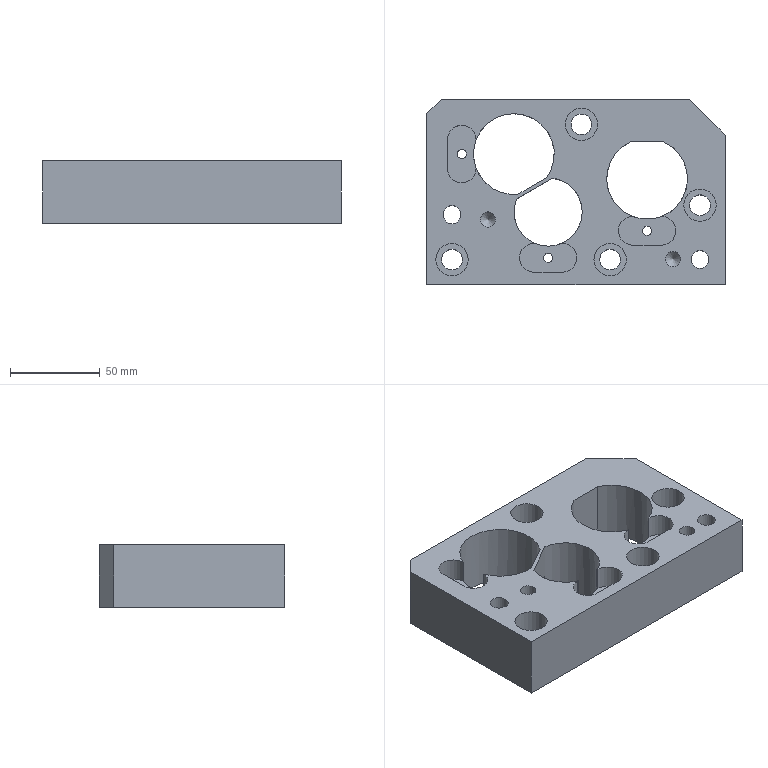Part | STEP file | lll_id4570_x_t | 1 solid | 49 faces | box 166 x 103.25 x 35 mm | volume 394773 mm3 | cylinder 24 | plane 23 | cone 2 | commonest cylinder face diameters 16 x6 11.509 x4 18.008 x4 5.206 x3 8.506 x2 10 x2
STEP:
#1=CARTESIAN_POINT('',(3308.367,-51.288,0.));
#2=VERTEX_POINT('',#1);
#3=CARTESIAN_POINT('',(3324.366,-51.364,0.));
#4=VERTEX_POINT('',#3);
#5=CARTESIAN_POINT('',(3316.367,-51.288,0.));
#6=DIRECTION('',(0.,0.,1.));
#7=DIRECTION('',(1.,0.,0.));
#8=AXIS2_PLACEMENT_3D('',#5,#6,#7);
#9=CIRCLE('',#8,8.);
#10=EDGE_CURVE('',#2,#4,#9,.T.);
#11=ORIENTED_EDGE('',*,*,#10,.F.);
#12=CARTESIAN_POINT('',(3308.367,-35.288,0.));
#13=VERTEX_POINT('',#12);
#14=CARTESIAN_POINT('',(3308.367,-54.25,0.));
#15=DIRECTION('',(0.,1.,0.));
#16=VECTOR('',#15,1.);
#17=LINE('',#14,#16);
#18=EDGE_CURVE('',#2,#13,#17,.T.);
#19=ORIENTED_EDGE('',*,*,#18,.T.);
#20=CARTESIAN_POINT('',(3324.366,-35.211,0.));
#21=VERTEX_POINT('',#20);
#22=CARTESIAN_POINT('',(3316.367,-35.288,0.));
#23=DIRECTION('',(0.,0.,1.));
#24=DIRECTION('',(1.,0.,0.));
#25=AXIS2_PLACEMENT_3D('',#22,#23,#24);
#26=CIRCLE('',#25,8.);
#27=EDGE_CURVE('',#21,#13,#26,.T.);
#28=ORIENTED_EDGE('',*,*,#27,.F.);
#29=CARTESIAN_POINT('',(3363.648,-56.404,0.));
#30=VERTEX_POINT('',#29);
#31=CARTESIAN_POINT('',(3345.367,-43.288,0.));
#32=DIRECTION('',(0.,0.,1.));
#33=DIRECTION('',(1.,0.,0.));
#34=AXIS2_PLACEMENT_3D('',#31,#32,#33);
#35=CIRCLE('',#34,22.5);
#36=EDGE_CURVE('',#30,#21,#35,.T.);
#37=ORIENTED_EDGE('',*,*,#36,.F.);
#38=CARTESIAN_POINT('',(3347.585,-65.678,0.));
#39=VERTEX_POINT('',#38);
#40=CARTESIAN_POINT('',(3355.617,-61.041,0.));
#41=DIRECTION('',(-0.866,-0.5,0.));
#42=VECTOR('',#41,1.);
#43=LINE('',#40,#42);
#44=EDGE_CURVE('',#30,#39,#43,.T.);
#45=ORIENTED_EDGE('',*,*,#44,.T.);
#46=CARTESIAN_POINT('',(3345.367,-43.288,0.));
#47=DIRECTION('',(0.,0.,1.));
#48=DIRECTION('',(1.,0.,0.));
#49=AXIS2_PLACEMENT_3D('',#46,#47,#48);
#50=CIRCLE('',#49,22.5);
#51=EDGE_CURVE('',#4,#39,#50,.T.);
#52=ORIENTED_EDGE('',*,*,#51,.F.);
#53=EDGE_LOOP('',(#11,#19,#28,#37,#45,#52));
#54=FACE_BOUND('',#53,.T.);
#55=CARTESIAN_POINT('',(3442.935,-12.75,0.));
#56=VERTEX_POINT('',#55);
#57=CARTESIAN_POINT('',(3304.935,-12.75,0.));
#58=VERTEX_POINT('',#57);
#59=CARTESIAN_POINT('',(3266.435,-12.75,0.));
#60=DIRECTION('',(-1.,0.,0.));
#61=VECTOR('',#60,1.);
#62=LINE('',#59,#61);
#63=EDGE_CURVE('',#56,#58,#62,.T.);
#64=ORIENTED_EDGE('',*,*,#63,.T.);
#65=CARTESIAN_POINT('',(3296.935,-20.75,0.));
#66=VERTEX_POINT('',#65);
#67=CARTESIAN_POINT('',(3179.435,-138.25,0.));
#68=DIRECTION('',(0.7071,0.7071,0.));
#69=VECTOR('',#68,1.);
#70=LINE('',#67,#69);
#71=EDGE_CURVE('',#66,#58,#70,.T.);
#72=ORIENTED_EDGE('',*,*,#71,.F.);
#73=CARTESIAN_POINT('',(3296.935,-116.,0.));
#74=VERTEX_POINT('',#73);
#75=CARTESIAN_POINT('',(3296.935,-215.25,0.));
#76=DIRECTION('',(0.,1.,0.));
#77=VECTOR('',#76,1.);
#78=LINE('',#75,#77);
#79=EDGE_CURVE('',#74,#66,#78,.T.);
#80=ORIENTED_EDGE('',*,*,#79,.F.);
#81=CARTESIAN_POINT('',(3462.935,-116.,0.));
#82=VERTEX_POINT('',#81);
#83=CARTESIAN_POINT('',(3266.435,-116.,0.));
#84=DIRECTION('',(-1.,0.,0.));
#85=VECTOR('',#84,1.);
#86=LINE('',#83,#85);
#87=EDGE_CURVE('',#82,#74,#86,.T.);
#88=ORIENTED_EDGE('',*,*,#87,.F.);
#89=CARTESIAN_POINT('',(3462.935,-32.75,0.));
#90=VERTEX_POINT('',#89);
#91=CARTESIAN_POINT('',(3462.935,-215.25,0.));
#92=DIRECTION('',(0.,1.,0.));
#93=VECTOR('',#92,1.);
#94=LINE('',#91,#93);
#95=EDGE_CURVE('',#82,#90,#94,.T.);
#96=ORIENTED_EDGE('',*,*,#95,.T.);
#97=CARTESIAN_POINT('',(3455.935,-25.75,0.));
#98=DIRECTION('',(0.7071,-0.7071,0.));
#99=VECTOR('',#98,1.);
#100=LINE('',#97,#99);
#101=EDGE_CURVE('',#56,#90,#100,.T.);
#102=ORIENTED_EDGE('',*,*,#101,.F.);
#103=EDGE_LOOP('',(#64,#72,#80,#88,#96,#102));
#104=FACE_BOUND('',#103,.T.);
#105=CARTESIAN_POINT('',(3319.939,-102.,0.));
#106=VERTEX_POINT('',#105);
#107=CARTESIAN_POINT('',(3310.935,-102.,0.));
#108=DIRECTION('',(0.,0.,-1.));
#109=DIRECTION('',(1.,0.,0.));
#110=AXIS2_PLACEMENT_3D('',#107,#108,#109);
#111=CIRCLE('',#110,9.004);
#112=EDGE_CURVE('',#106,#106,#111,.T.);
#113=ORIENTED_EDGE('',*,*,#112,.T.);
#114=EDGE_LOOP('',(#113));
#115=FACE_BOUND('',#114,.T.);
#116=CARTESIAN_POINT('',(3315.935,-77.,0.));
#117=VERTEX_POINT('',#116);
#118=CARTESIAN_POINT('',(3310.935,-77.,0.));
#119=DIRECTION('',(0.,0.,-1.));
#120=DIRECTION('',(1.,0.,0.));
#121=AXIS2_PLACEMENT_3D('',#118,#119,#120);
#122=CIRCLE('',#121,5.);
#123=EDGE_CURVE('',#117,#117,#122,.T.);
#124=ORIENTED_EDGE('',*,*,#123,.T.);
#125=EDGE_LOOP('',(#124));
#126=FACE_BOUND('',#125,.T.);
#127=CARTESIAN_POINT('',(3335.188,-79.75,0.));
#128=VERTEX_POINT('',#127);
#129=CARTESIAN_POINT('',(3330.935,-79.75,0.));
#130=DIRECTION('',(0.,0.,-1.));
#131=DIRECTION('',(1.,0.,0.));
#132=AXIS2_PLACEMENT_3D('',#129,#130,#131);
#133=CIRCLE('',#132,4.253);
#134=EDGE_CURVE('',#128,#128,#133,.T.);
#135=ORIENTED_EDGE('',*,*,#134,.T.);
#136=EDGE_LOOP('',(#135));
#137=FACE_BOUND('',#136,.T.);
#138=CARTESIAN_POINT('',(3391.939,-26.75,0.));
#139=VERTEX_POINT('',#138);
#140=CARTESIAN_POINT('',(3382.935,-26.75,0.));
#141=DIRECTION('',(0.,0.,-1.));
#142=DIRECTION('',(1.,0.,0.));
#143=AXIS2_PLACEMENT_3D('',#140,#141,#142);
#144=CIRCLE('',#143,9.004);
#145=EDGE_CURVE('',#139,#139,#144,.T.);
#146=ORIENTED_EDGE('',*,*,#145,.T.);
#147=EDGE_LOOP('',(#146));
#148=FACE_BOUND('',#147,.T.);
#149=CARTESIAN_POINT('',(3457.939,-71.75,0.));
#150=VERTEX_POINT('',#149);
#151=CARTESIAN_POINT('',(3448.935,-71.75,0.));
#152=DIRECTION('',(0.,0.,-1.));
#153=DIRECTION('',(1.,0.,0.));
#154=AXIS2_PLACEMENT_3D('',#151,#152,#153);
#155=CIRCLE('',#154,9.004);
#156=EDGE_CURVE('',#150,#150,#155,.T.);
#157=ORIENTED_EDGE('',*,*,#156,.T.);
#158=EDGE_LOOP('',(#157));
#159=FACE_BOUND('',#158,.T.);
#160=CARTESIAN_POINT('',(3453.935,-102.,0.));
#161=VERTEX_POINT('',#160);
#162=CARTESIAN_POINT('',(3448.935,-102.,0.));
#163=DIRECTION('',(0.,0.,-1.));
#164=DIRECTION('',(1.,0.,0.));
#165=AXIS2_PLACEMENT_3D('',#162,#163,#164);
#166=CIRCLE('',#165,5.);
#167=EDGE_CURVE('',#161,#161,#166,.T.);
#168=ORIENTED_EDGE('',*,*,#167,.T.);
#169=EDGE_LOOP('',(#168));
#170=FACE_BOUND('',#169,.T.);
#171=CARTESIAN_POINT('',(3407.939,-102.,0.));
#172=VERTEX_POINT('',#171);
#173=CARTESIAN_POINT('',(3398.935,-102.,0.));
#174=DIRECTION('',(0.,0.,-1.));
#175=DIRECTION('',(1.,0.,0.));
#176=AXIS2_PLACEMENT_3D('',#173,#174,#175);
#177=CIRCLE('',#176,9.004);
#178=EDGE_CURVE('',#172,#172,#177,.T.);
#179=ORIENTED_EDGE('',*,*,#178,.T.);
#180=EDGE_LOOP('',(#179));
#181=FACE_BOUND('',#180,.T.);
#182=CARTESIAN_POINT('',(3438.188,-101.75,0.));
#183=VERTEX_POINT('',#182);
#184=CARTESIAN_POINT('',(3433.935,-101.75,0.));
#185=DIRECTION('',(0.,0.,-1.));
#186=DIRECTION('',(1.,0.,0.));
#187=AXIS2_PLACEMENT_3D('',#184,#185,#186);
#188=CIRCLE('',#187,4.253);
#189=EDGE_CURVE('',#183,#183,#188,.T.);
#190=ORIENTED_EDGE('',*,*,#189,.T.);
#191=EDGE_LOOP('',(#190));
#192=FACE_BOUND('',#191,.T.);
#193=CARTESIAN_POINT('',(3427.5,-94.,0.));
#194=VERTEX_POINT('',#193);
#195=CARTESIAN_POINT('',(3427.577,-78.,0.));
#196=VERTEX_POINT('',#195);
#197=CARTESIAN_POINT('',(3427.5,-86.,0.));
#198=DIRECTION('',(0.,0.,1.));
#199=DIRECTION('',(0.,1.,0.));
#200=AXIS2_PLACEMENT_3D('',#197,#198,#199);
#201=CIRCLE('',#200,8.);
#202=EDGE_CURVE('',#194,#196,#201,.T.);
#203=ORIENTED_EDGE('',*,*,#202,.F.);
#204=CARTESIAN_POINT('',(3411.5,-94.,0.));
#205=VERTEX_POINT('',#204);
#206=CARTESIAN_POINT('',(3430.462,-94.,0.));
#207=DIRECTION('',(-1.,0.,0.));
#208=VECTOR('',#207,1.);
#209=LINE('',#206,#208);
#210=EDGE_CURVE('',#194,#205,#209,.T.);
#211=ORIENTED_EDGE('',*,*,#210,.T.);
#212=CARTESIAN_POINT('',(3411.423,-78.,0.));
#213=VERTEX_POINT('',#212);
#214=CARTESIAN_POINT('',(3411.5,-86.,0.));
#215=DIRECTION('',(0.,0.,1.));
#216=DIRECTION('',(0.,1.,0.));
#217=AXIS2_PLACEMENT_3D('',#214,#215,#216);
#218=CIRCLE('',#217,8.);
#219=EDGE_CURVE('',#213,#205,#218,.T.);
#220=ORIENTED_EDGE('',*,*,#219,.F.);
#221=CARTESIAN_POINT('',(3410.226,-36.5,0.));
#222=VERTEX_POINT('',#221);
#223=CARTESIAN_POINT('',(3419.5,-57.,0.));
#224=DIRECTION('',(0.,0.,-1.));
#225=DIRECTION('',(1.,0.,0.));
#226=AXIS2_PLACEMENT_3D('',#223,#224,#225);
#227=CIRCLE('',#226,22.5);
#228=EDGE_CURVE('',#213,#222,#227,.T.);
#229=ORIENTED_EDGE('',*,*,#228,.T.);
#230=CARTESIAN_POINT('',(3428.774,-36.5,0.));
#231=VERTEX_POINT('',#230);
#232=CARTESIAN_POINT('',(3419.5,-36.5,0.));
#233=DIRECTION('',(1.,0.,0.));
#234=VECTOR('',#233,1.);
#235=LINE('',#232,#234);
#236=EDGE_CURVE('',#222,#231,#235,.T.);
#237=ORIENTED_EDGE('',*,*,#236,.T.);
#238=CARTESIAN_POINT('',(3419.5,-57.,0.));
#239=DIRECTION('',(0.,0.,-1.));
#240=DIRECTION('',(1.,0.,0.));
#241=AXIS2_PLACEMENT_3D('',#238,#239,#240);
#242=CIRCLE('',#241,22.5);
#243=EDGE_CURVE('',#231,#196,#242,.T.);
#244=ORIENTED_EDGE('',*,*,#243,.T.);
#245=EDGE_LOOP('',(#203,#211,#220,#229,#237,#244));
#246=FACE_BOUND('',#245,.T.);
#247=CARTESIAN_POINT('',(3371.834,-93.,0.));
#248=VERTEX_POINT('',#247);
#249=CARTESIAN_POINT('',(3367.034,-56.679,0.));
#250=VERTEX_POINT('',#249);
#251=CARTESIAN_POINT('',(3364.435,-75.5,0.));
#252=DIRECTION('',(0.,0.,1.));
#253=DIRECTION('',(-1.,0.,0.));
#254=AXIS2_PLACEMENT_3D('',#251,#252,#253);
#255=CIRCLE('',#254,19.);
#256=EDGE_CURVE('',#248,#250,#255,.T.);
#257=ORIENTED_EDGE('',*,*,#256,.F.);
#258=CARTESIAN_POINT('',(3372.435,-93.,0.));
#259=VERTEX_POINT('',#258);
#260=CARTESIAN_POINT('',(3375.397,-93.,0.));
#261=DIRECTION('',(1.,0.,0.));
#262=VECTOR('',#261,1.);
#263=LINE('',#260,#262);
#264=EDGE_CURVE('',#248,#259,#263,.T.);
#265=ORIENTED_EDGE('',*,*,#264,.T.);
#266=CARTESIAN_POINT('',(3372.435,-109.,0.));
#267=VERTEX_POINT('',#266);
#268=CARTESIAN_POINT('',(3372.435,-101.,0.));
#269=DIRECTION('',(0.,0.,1.));
#270=DIRECTION('',(0.,1.,0.));
#271=AXIS2_PLACEMENT_3D('',#268,#269,#270);
#272=CIRCLE('',#271,8.);
#273=EDGE_CURVE('',#267,#259,#272,.T.);
#274=ORIENTED_EDGE('',*,*,#273,.F.);
#275=CARTESIAN_POINT('',(3356.435,-109.,0.));
#276=VERTEX_POINT('',#275);
#277=CARTESIAN_POINT('',(3375.397,-109.,0.));
#278=DIRECTION('',(-1.,0.,0.));
#279=VECTOR('',#278,1.);
#280=LINE('',#277,#279);
#281=EDGE_CURVE('',#267,#276,#280,.T.);
#282=ORIENTED_EDGE('',*,*,#281,.T.);
#283=CARTESIAN_POINT('',(3356.435,-93.,0.));
#284=VERTEX_POINT('',#283);
#285=CARTESIAN_POINT('',(3356.435,-101.,0.));
#286=DIRECTION('',(0.,0.,1.));
#287=DIRECTION('',(0.,1.,0.));
#288=AXIS2_PLACEMENT_3D('',#285,#286,#287);
#289=CIRCLE('',#288,8.);
#290=EDGE_CURVE('',#284,#276,#289,.T.);
#291=ORIENTED_EDGE('',*,*,#290,.F.);
#292=CARTESIAN_POINT('',(3357.036,-93.,0.));
#293=VERTEX_POINT('',#292);
#294=CARTESIAN_POINT('',(3375.397,-93.,0.));
#295=DIRECTION('',(1.,0.,0.));
#296=VECTOR('',#295,1.);
#297=LINE('',#294,#296);
#298=EDGE_CURVE('',#284,#293,#297,.T.);
#299=ORIENTED_EDGE('',*,*,#298,.T.);
#300=CARTESIAN_POINT('',(3346.835,-68.341,0.));
#301=VERTEX_POINT('',#300);
#302=CARTESIAN_POINT('',(3364.435,-75.5,0.));
#303=DIRECTION('',(0.,0.,1.));
#304=DIRECTION('',(-1.,0.,0.));
#305=AXIS2_PLACEMENT_3D('',#302,#303,#304);
#306=CIRCLE('',#305,19.);
#307=EDGE_CURVE('',#301,#293,#306,.T.);
#308=ORIENTED_EDGE('',*,*,#307,.F.);
#309=CARTESIAN_POINT('',(3356.935,-62.51,0.));
#310=DIRECTION('',(-0.866,-0.5,0.));
#311=VECTOR('',#310,1.);
#312=LINE('',#309,#311);
#313=EDGE_CURVE('',#250,#301,#312,.T.);
#314=ORIENTED_EDGE('',*,*,#313,.F.);
#315=EDGE_LOOP('',(#257,#265,#274,#282,#291,#299,#308,#314));
#316=FACE_BOUND('',#315,.T.);
#317=CARTESIAN_POINT('',(3266.435,-215.25,0.));
#318=DIRECTION('',(0.,0.,1.));
#319=DIRECTION('',(-1.,0.,0.));
#320=AXIS2_PLACEMENT_3D('',#317,#318,#319);
#321=PLANE('',#320);
#322=ADVANCED_FACE('',(#54,#104,#115,#126,#137,#148,#159,#170,#181,#192,#246,#316),#321,.T.);
#323=CARTESIAN_POINT('',(3371.834,-93.,-13.));
#324=VERTEX_POINT('',#323);
#325=CARTESIAN_POINT('',(3371.834,-93.,-17.5));
#326=DIRECTION('',(0.,0.,-1.));
#327=VECTOR('',#326,1.);
#328=LINE('',#325,#327);
#329=EDGE_CURVE('',#248,#324,#328,.T.);
#330=ORIENTED_EDGE('',*,*,#329,.F.);
#331=ORIENTED_EDGE('',*,*,#256,.T.);
#332=CARTESIAN_POINT('',(3367.034,-56.679,-35.));
#333=VERTEX_POINT('',#332);
#334=CARTESIAN_POINT('',(3367.034,-56.679,-15.));
#335=DIRECTION('',(0.,0.,1.));
#336=VECTOR('',#335,1.);
#337=LINE('',#334,#336);
#338=EDGE_CURVE('',#333,#250,#337,.T.);
#339=ORIENTED_EDGE('',*,*,#338,.F.);
#340=CARTESIAN_POINT('',(3346.835,-68.341,-35.));
#341=VERTEX_POINT('',#340);
#342=CARTESIAN_POINT('',(3364.435,-75.5,-35.));
#343=DIRECTION('',(0.,0.,1.));
#344=DIRECTION('',(-1.,0.,0.));
#345=AXIS2_PLACEMENT_3D('',#342,#343,#344);
#346=CIRCLE('',#345,19.);
#347=EDGE_CURVE('',#341,#333,#346,.T.);
#348=ORIENTED_EDGE('',*,*,#347,.F.);
#349=CARTESIAN_POINT('',(3346.835,-68.341,-15.));
#350=DIRECTION('',(0.,0.,-1.));
#351=VECTOR('',#350,1.);
#352=LINE('',#349,#351);
#353=EDGE_CURVE('',#301,#341,#352,.T.);
#354=ORIENTED_EDGE('',*,*,#353,.F.);
#355=ORIENTED_EDGE('',*,*,#307,.T.);
#356=CARTESIAN_POINT('',(3357.036,-93.,-13.));
#357=VERTEX_POINT('',#356);
#358=CARTESIAN_POINT('',(3357.036,-93.,-17.5));
#359=DIRECTION('',(0.,0.,1.));
#360=VECTOR('',#359,1.);
#361=LINE('',#358,#360);
#362=EDGE_CURVE('',#357,#293,#361,.T.);
#363=ORIENTED_EDGE('',*,*,#362,.F.);
#364=CARTESIAN_POINT('',(3364.435,-75.5,-13.));
#365=DIRECTION('',(0.,0.,-1.));
#366=DIRECTION('',(1.,0.,0.));
#367=AXIS2_PLACEMENT_3D('',#364,#365,#366);
#368=CIRCLE('',#367,19.);
#369=EDGE_CURVE('',#324,#357,#368,.T.);
#370=ORIENTED_EDGE('',*,*,#369,.F.);
#371=EDGE_LOOP('',(#330,#331,#339,#348,#354,#355,#363,#370));
#372=FACE_OUTER_BOUND('',#371,.T.);
#373=CARTESIAN_POINT('',(3364.435,-75.5,-17.5));
#374=DIRECTION('',(0.,0.,1.));
#375=DIRECTION('',(0.,1.,0.));
#376=AXIS2_PLACEMENT_3D('',#373,#374,#375);
#377=CYLINDRICAL_SURFACE('',#376,19.);
#378=ADVANCED_FACE('',(#372),#377,.F.);
#379=CARTESIAN_POINT('',(3313.764,-43.288,-35.));
#380=VERTEX_POINT('',#379);
#381=CARTESIAN_POINT('',(3316.367,-43.288,-35.));
#382=DIRECTION('',(0.,0.,-1.));
#383=DIRECTION('',(-1.,0.,0.));
#384=AXIS2_PLACEMENT_3D('',#381,#382,#383);
#385=CIRCLE('',#384,2.603);
#386=EDGE_CURVE('',#380,#380,#385,.T.);
#387=ORIENTED_EDGE('',*,*,#386,.F.);
#388=EDGE_LOOP('',(#387));
#389=FACE_BOUND('',#388,.T.);
#390=CARTESIAN_POINT('',(3364.435,-103.603,-35.));
#391=VERTEX_POINT('',#390);
#392=CARTESIAN_POINT('',(3364.435,-101.,-35.));
#393=DIRECTION('',(0.,0.,-1.));
#394=DIRECTION('',(0.,-1.,0.));
#395=AXIS2_PLACEMENT_3D('',#392,#393,#394);
#396=CIRCLE('',#395,2.603);
#397=EDGE_CURVE('',#391,#391,#396,.T.);
#398=ORIENTED_EDGE('',*,*,#397,.F.);
#399=EDGE_LOOP('',(#398));
#400=FACE_BOUND('',#399,.T.);
#401=CARTESIAN_POINT('',(3419.5,-88.603,-35.));
#402=VERTEX_POINT('',#401);
#403=CARTESIAN_POINT('',(3419.5,-86.,-35.));
#404=DIRECTION('',(0.,0.,-1.));
#405=DIRECTION('',(0.,-1.,0.));
#406=AXIS2_PLACEMENT_3D('',#403,#404,#405);
#407=CIRCLE('',#406,2.603);
#408=EDGE_CURVE('',#402,#402,#407,.T.);
#409=ORIENTED_EDGE('',*,*,#408,.F.);
#410=EDGE_LOOP('',(#409));
#411=FACE_BOUND('',#410,.T.);
#412=CARTESIAN_POINT('',(3443.181,-71.75,-35.));
#413=VERTEX_POINT('',#412);
#414=CARTESIAN_POINT('',(3448.935,-71.75,-35.));
#415=DIRECTION('',(0.,0.,1.));
#416=DIRECTION('',(-1.,0.,0.));
#417=AXIS2_PLACEMENT_3D('',#414,#415,#416);
#418=CIRCLE('',#417,5.755);
#419=EDGE_CURVE('',#413,#413,#418,.T.);
#420=ORIENTED_EDGE('',*,*,#419,.T.);
#421=EDGE_LOOP('',(#420));
#422=FACE_BOUND('',#421,.T.);
#423=CARTESIAN_POINT('',(3393.181,-102.,-35.));
#424=VERTEX_POINT('',#423);
#425=CARTESIAN_POINT('',(3398.935,-102.,-35.));
#426=DIRECTION('',(0.,0.,1.));
#427=DIRECTION('',(-1.,0.,0.));
#428=AXIS2_PLACEMENT_3D('',#425,#426,#427);
#429=CIRCLE('',#428,5.755);
#430=EDGE_CURVE('',#424,#424,#429,.T.);
#431=ORIENTED_EDGE('',*,*,#430,.T.);
#432=EDGE_LOOP('',(#431));
#433=FACE_BOUND('',#432,.T.);
#434=CARTESIAN_POINT('',(3377.181,-26.75,-35.));
#435=VERTEX_POINT('',#434);
#436=CARTESIAN_POINT('',(3382.935,-26.75,-35.));
#437=DIRECTION('',(0.,0.,1.));
#438=DIRECTION('',(-1.,0.,0.));
#439=AXIS2_PLACEMENT_3D('',#436,#437,#438);
#440=CIRCLE('',#439,5.755);
#441=EDGE_CURVE('',#435,#435,#440,.T.);
#442=ORIENTED_EDGE('',*,*,#441,.T.);
#443=EDGE_LOOP('',(#442));
#444=FACE_BOUND('',#443,.T.);
#445=CARTESIAN_POINT('',(3305.935,-77.,-35.));
#446=VERTEX_POINT('',#445);
#447=CARTESIAN_POINT('',(3310.935,-77.,-35.));
#448=DIRECTION('',(0.,0.,1.));
#449=DIRECTION('',(-1.,0.,0.));
#450=AXIS2_PLACEMENT_3D('',#447,#448,#449);
#451=CIRCLE('',#450,5.);
#452=EDGE_CURVE('',#446,#446,#451,.T.);
#453=ORIENTED_EDGE('',*,*,#452,.T.);
#454=EDGE_LOOP('',(#453));
#455=FACE_BOUND('',#454,.T.);
#456=CARTESIAN_POINT('',(3305.181,-102.,-35.));
#457=VERTEX_POINT('',#456);
#458=CARTESIAN_POINT('',(3310.935,-102.,-35.));
#459=DIRECTION('',(0.,0.,1.));
#460=DIRECTION('',(-1.,0.,0.));
#461=AXIS2_PLACEMENT_3D('',#458,#459,#460);
#462=CIRCLE('',#461,5.755);
#463=EDGE_CURVE('',#457,#457,#462,.T.);
#464=ORIENTED_EDGE('',*,*,#463,.T.);
#465=EDGE_LOOP('',(#464));
#466=FACE_BOUND('',#465,.T.);
#467=CARTESIAN_POINT('',(3304.935,-12.75,-35.));
#468=VERTEX_POINT('',#467);
#469=CARTESIAN_POINT('',(3442.935,-12.75,-35.));
#470=VERTEX_POINT('',#469);
#471=CARTESIAN_POINT('',(3266.435,-12.75,-35.));
#472=DIRECTION('',(1.,0.,0.));
#473=VECTOR('',#472,1.);
#474=LINE('',#471,#473);
#475=EDGE_CURVE('',#468,#470,#474,.T.);
#476=ORIENTED_EDGE('',*,*,#475,.T.);
#477=CARTESIAN_POINT('',(3462.935,-32.75,-35.));
#478=VERTEX_POINT('',#477);
#479=CARTESIAN_POINT('',(3455.935,-25.75,-35.));
#480=DIRECTION('',(-0.7071,0.7071,0.));
#481=VECTOR('',#480,1.);
#482=LINE('',#479,#481);
#483=EDGE_CURVE('',#478,#470,#482,.T.);
#484=ORIENTED_EDGE('',*,*,#483,.F.);
#485=CARTESIAN_POINT('',(3462.935,-116.,-35.));
#486=VERTEX_POINT('',#485);
#487=CARTESIAN_POINT('',(3462.935,-215.25,-35.));
#488=DIRECTION('',(0.,-1.,0.));
#489=VECTOR('',#488,1.);
#490=LINE('',#487,#489);
#491=EDGE_CURVE('',#478,#486,#490,.T.);
#492=ORIENTED_EDGE('',*,*,#491,.T.);
#493=CARTESIAN_POINT('',(3296.935,-116.,-35.));
#494=VERTEX_POINT('',#493);
#495=CARTESIAN_POINT('',(3266.435,-116.,-35.));
#496=DIRECTION('',(-1.,0.,0.));
#497=VECTOR('',#496,1.);
#498=LINE('',#495,#497);
#499=EDGE_CURVE('',#486,#494,#498,.T.);
#500=ORIENTED_EDGE('',*,*,#499,.T.);
#501=CARTESIAN_POINT('',(3296.935,-20.75,-35.));
#502=VERTEX_POINT('',#501);
#503=CARTESIAN_POINT('',(3296.935,-215.25,-35.));
#504=DIRECTION('',(0.,1.,0.));
#505=VECTOR('',#504,1.);
#506=LINE('',#503,#505);
#507=EDGE_CURVE('',#494,#502,#506,.T.);
#508=ORIENTED_EDGE('',*,*,#507,.T.);
#509=CARTESIAN_POINT('',(3179.435,-138.25,-35.));
#510=DIRECTION('',(-0.7071,-0.7071,0.));
#511=VECTOR('',#510,1.);
#512=LINE('',#509,#511);
#513=EDGE_CURVE('',#468,#502,#512,.T.);
#514=ORIENTED_EDGE('',*,*,#513,.F.);
#515=EDGE_LOOP('',(#476,#484,#492,#500,#508,#514));
#516=FACE_BOUND('',#515,.T.);
#517=CARTESIAN_POINT('',(3443.935,-102.,-35.));
#518=VERTEX_POINT('',#517);
#519=CARTESIAN_POINT('',(3448.935,-102.,-35.));
#520=DIRECTION('',(0.,0.,1.));
#521=DIRECTION('',(-1.,0.,0.));
#522=AXIS2_PLACEMENT_3D('',#519,#520,#521);
#523=CIRCLE('',#522,5.);
#524=EDGE_CURVE('',#518,#518,#523,.T.);
#525=ORIENTED_EDGE('',*,*,#524,.T.);
#526=EDGE_LOOP('',(#525));
#527=FACE_BOUND('',#526,.T.);
#528=CARTESIAN_POINT('',(3222.922,-139.882,-35.));
#529=DIRECTION('',(0.866,0.5,0.));
#530=VECTOR('',#529,1.);
#531=LINE('',#528,#530);
#532=EDGE_CURVE('',#341,#333,#531,.T.);
#533=ORIENTED_EDGE('',*,*,#532,.F.);
#534=ORIENTED_EDGE('',*,*,#347,.T.);
#535=EDGE_LOOP('',(#533,#534));
#536=FACE_BOUND('',#535,.T.);
#537=CARTESIAN_POINT('',(3363.648,-56.404,-35.));
#538=VERTEX_POINT('',#537);
#539=CARTESIAN_POINT('',(3347.585,-65.678,-35.));
#540=VERTEX_POINT('',#539);
#541=CARTESIAN_POINT('',(3221.956,-138.21,-35.));
#542=DIRECTION('',(-0.866,-0.5,0.));
#543=VECTOR('',#542,1.);
#544=LINE('',#541,#543);
#545=EDGE_CURVE('',#538,#540,#544,.T.);
#546=ORIENTED_EDGE('',*,*,#545,.F.);
#547=CARTESIAN_POINT('',(3345.367,-43.288,-35.));
#548=DIRECTION('',(0.,0.,-1.));
#549=DIRECTION('',(-1.,0.,0.));
#550=AXIS2_PLACEMENT_3D('',#547,#548,#549);
#551=CIRCLE('',#550,22.5);
#552=EDGE_CURVE('',#540,#538,#551,.T.);
#553=ORIENTED_EDGE('',*,*,#552,.F.);
#554=EDGE_LOOP('',(#546,#553));
#555=FACE_BOUND('',#554,.T.);
#556=CARTESIAN_POINT('',(3428.774,-36.5,-35.));
#557=VERTEX_POINT('',#556);
#558=CARTESIAN_POINT('',(3410.226,-36.5,-35.));
#559=VERTEX_POINT('',#558);
#560=CARTESIAN_POINT('',(3419.5,-36.5,-35.));
#561=DIRECTION('',(-1.,0.,0.));
#562=VECTOR('',#561,1.);
#563=LINE('',#560,#562);
#564=EDGE_CURVE('',#557,#559,#563,.T.);
#565=ORIENTED_EDGE('',*,*,#564,.T.);
#566=CARTESIAN_POINT('',(3419.5,-57.,-35.));
#567=DIRECTION('',(0.,0.,-1.));
#568=DIRECTION('',(-1.,0.,0.));
#569=AXIS2_PLACEMENT_3D('',#566,#567,#568);
#570=CIRCLE('',#569,22.5);
#571=EDGE_CURVE('',#557,#559,#570,.T.);
#572=ORIENTED_EDGE('',*,*,#571,.F.);
#573=EDGE_LOOP('',(#565,#572));
#574=FACE_BOUND('',#573,.T.);
#575=CARTESIAN_POINT('',(3266.435,-215.25,-35.));
#576=DIRECTION('',(0.,0.,-1.));
#577=DIRECTION('',(1.,0.,0.));
#578=AXIS2_PLACEMENT_3D('',#575,#576,#577);
#579=PLANE('',#578);
#580=ADVANCED_FACE('',(#389,#400,#411,#422,#433,#444,#455,#466,#516,#527,#536,#555,#574),#579,.T.);
#581=ORIENTED_EDGE('',*,*,#353,.T.);
#582=ORIENTED_EDGE('',*,*,#532,.T.);
#583=ORIENTED_EDGE('',*,*,#338,.T.);
#584=ORIENTED_EDGE('',*,*,#313,.T.);
#585=EDGE_LOOP('',(#581,#582,#583,#584));
#586=FACE_OUTER_BOUND('',#585,.T.);
#587=CARTESIAN_POINT('',(3356.935,-62.51,-32.5));
#588=DIRECTION('',(-0.5,0.866,0.));
#589=DIRECTION('',(-0.866,-0.5,0.));
#590=AXIS2_PLACEMENT_3D('',#587,#588,#589);
#591=PLANE('',#590);
#592=ADVANCED_FACE('',(#586),#591,.F.);
#593=CARTESIAN_POINT('',(3363.648,-56.404,0.00001711));
#594=DIRECTION('',(0.,0.,-1.));
#595=VECTOR('',#594,1.);
#596=LINE('',#593,#595);
#597=EDGE_CURVE('',#30,#538,#596,.T.);
#598=ORIENTED_EDGE('',*,*,#597,.T.);
#599=ORIENTED_EDGE('',*,*,#545,.T.);
#600=CARTESIAN_POINT('',(3347.585,-65.678,-30.));
#601=DIRECTION('',(0.,0.,1.));
#602=VECTOR('',#601,1.);
#603=LINE('',#600,#602);
#604=EDGE_CURVE('',#540,#39,#603,.T.);
#605=ORIENTED_EDGE('',*,*,#604,.T.);
#606=ORIENTED_EDGE('',*,*,#44,.F.);
#607=EDGE_LOOP('',(#598,#599,#605,#606));
#608=FACE_OUTER_BOUND('',#607,.T.);
#609=CARTESIAN_POINT('',(3355.617,-61.041,-32.5));
#610=DIRECTION('',(0.5,-0.866,0.));
#611=DIRECTION('',(0.866,0.5,0.));
#612=AXIS2_PLACEMENT_3D('',#609,#610,#611);
#613=PLANE('',#612);
#614=ADVANCED_FACE('',(#608),#613,.F.);
#615=ORIENTED_EDGE('',*,*,#475,.F.);
#616=CARTESIAN_POINT('',(3304.935,-12.75,-35.));
#617=DIRECTION('',(0.,0.,-1.));
#618=VECTOR('',#617,1.);
#619=LINE('',#616,#618);
#620=EDGE_CURVE('',#58,#468,#619,.T.);
#621=ORIENTED_EDGE('',*,*,#620,.F.);
#622=ORIENTED_EDGE('',*,*,#63,.F.);
#623=CARTESIAN_POINT('',(3442.935,-12.75,-32.));
#624=DIRECTION('',(0.,0.,1.));
#625=VECTOR('',#624,1.);
#626=LINE('',#623,#625);
#627=EDGE_CURVE('',#470,#56,#626,.T.);
#628=ORIENTED_EDGE('',*,*,#627,.F.);
#629=EDGE_LOOP('',(#615,#621,#622,#628));
#630=FACE_OUTER_BOUND('',#629,.T.);
#631=CARTESIAN_POINT('',(3266.435,-12.75,-32.));
#632=DIRECTION('',(0.,1.,0.));
#633=DIRECTION('',(0.,0.,1.));
#634=AXIS2_PLACEMENT_3D('',#631,#632,#633);
#635=PLANE('',#634);
#636=ADVANCED_FACE('',(#630),#635,.T.);
#637=ORIENTED_EDGE('',*,*,#95,.F.);
#638=CARTESIAN_POINT('',(3462.935,-116.,-32.));
#639=DIRECTION('',(0.,0.,1.));
#640=VECTOR('',#639,1.);
#641=LINE('',#638,#640);
#642=EDGE_CURVE('',#486,#82,#641,.T.);
#643=ORIENTED_EDGE('',*,*,#642,.F.);
#644=ORIENTED_EDGE('',*,*,#491,.F.);
#645=CARTESIAN_POINT('',(3462.935,-32.75,-32.));
#646=DIRECTION('',(0.,0.,-1.));
#647=VECTOR('',#646,1.);
#648=LINE('',#645,#647);
#649=EDGE_CURVE('',#90,#478,#648,.T.);
#650=ORIENTED_EDGE('',*,*,#649,.F.);
#651=EDGE_LOOP('',(#637,#643,#644,#650));
#652=FACE_OUTER_BOUND('',#651,.T.);
#653=CARTESIAN_POINT('',(3462.935,-215.25,-32.));
#654=DIRECTION('',(1.,0.,0.));
#655=DIRECTION('',(0.,0.,1.));
#656=AXIS2_PLACEMENT_3D('',#653,#654,#655);
#657=PLANE('',#656);
#658=ADVANCED_FACE('',(#652),#657,.T.);
#659=ORIENTED_EDGE('',*,*,#499,.F.);
#660=ORIENTED_EDGE('',*,*,#642,.T.);
#661=ORIENTED_EDGE('',*,*,#87,.T.);
#662=CARTESIAN_POINT('',(3296.935,-116.,-17.5));
#663=DIRECTION('',(0.,0.,-1.));
#664=VECTOR('',#663,1.);
#665=LINE('',#662,#664);
#666=EDGE_CURVE('',#74,#494,#665,.T.);
#667=ORIENTED_EDGE('',*,*,#666,.T.);
#668=EDGE_LOOP('',(#659,#660,#661,#667));
#669=FACE_OUTER_BOUND('',#668,.T.);
#670=CARTESIAN_POINT('',(3384.935,-116.,-17.5));
#671=DIRECTION('',(0.,1.,0.));
#672=DIRECTION('',(0.,0.,-1.));
#673=AXIS2_PLACEMENT_3D('',#670,#671,#672);
#674=PLANE('',#673);
#675=ADVANCED_FACE('',(#669),#674,.F.);
#676=ORIENTED_EDGE('',*,*,#507,.F.);
#677=ORIENTED_EDGE('',*,*,#666,.F.);
#678=ORIENTED_EDGE('',*,*,#79,.T.);
#679=CARTESIAN_POINT('',(3296.935,-20.75,0.));
#680=DIRECTION('',(0.,0.,1.));
#681=VECTOR('',#680,1.);
#682=LINE('',#679,#681);
#683=EDGE_CURVE('',#502,#66,#682,.T.);
#684=ORIENTED_EDGE('',*,*,#683,.F.);
#685=EDGE_LOOP('',(#676,#677,#678,#684));
#686=FACE_OUTER_BOUND('',#685,.T.);
#687=CARTESIAN_POINT('',(3296.935,-62.,-17.5));
#688=DIRECTION('',(1.,0.,0.));
#689=DIRECTION('',(0.,0.,-1.));
#690=AXIS2_PLACEMENT_3D('',#687,#688,#689);
#691=PLANE('',#690);
#692=ADVANCED_FACE('',(#686),#691,.F.);
#693=ORIENTED_EDGE('',*,*,#463,.F.);
#694=EDGE_LOOP('',(#693));
#695=FACE_BOUND('',#694,.T.);
#696=CARTESIAN_POINT('',(3305.181,-102.,-13.));
#697=VERTEX_POINT('',#696);
#698=CARTESIAN_POINT('',(3310.935,-102.,-13.));
#699=DIRECTION('',(0.,0.,1.));
#700=DIRECTION('',(-1.,0.,0.));
#701=AXIS2_PLACEMENT_3D('',#698,#699,#700);
#702=CIRCLE('',#701,5.755);
#703=EDGE_CURVE('',#697,#697,#702,.T.);
#704=ORIENTED_EDGE('',*,*,#703,.T.);
#705=EDGE_LOOP('',(#704));
#706=FACE_BOUND('',#705,.T.);
#707=CARTESIAN_POINT('',(3310.935,-102.,2.));
#708=DIRECTION('',(0.,0.,-1.));
#709=DIRECTION('',(1.,0.,0.));
#710=AXIS2_PLACEMENT_3D('',#707,#708,#709);
#711=CYLINDRICAL_SURFACE('',#710,5.755);
#712=ADVANCED_FACE('',(#695,#706),#711,.F.);
#713=ORIENTED_EDGE('',*,*,#703,.F.);
#714=EDGE_LOOP('',(#713));
#715=FACE_BOUND('',#714,.T.);
#716=CARTESIAN_POINT('',(3319.939,-102.,-13.));
#717=VERTEX_POINT('',#716);
#718=CARTESIAN_POINT('',(3310.935,-102.,-13.));
#719=DIRECTION('',(0.,0.,1.));
#720=DIRECTION('',(1.,0.,0.));
#721=AXIS2_PLACEMENT_3D('',#718,#719,#720);
#722=CIRCLE('',#721,9.004);
#723=EDGE_CURVE('',#717,#717,#722,.T.);
#724=ORIENTED_EDGE('',*,*,#723,.T.);
#725=EDGE_LOOP('',(#724));
#726=FACE_BOUND('',#725,.T.);
#727=CARTESIAN_POINT('',(3310.935,-102.,-13.));
#728=DIRECTION('',(0.,0.,-1.));
#729=DIRECTION('',(-1.,0.,0.));
#730=AXIS2_PLACEMENT_3D('',#727,#728,#729);
#731=PLANE('',#730);
#732=ADVANCED_FACE('',(#715,#726),#731,.F.);
#733=ORIENTED_EDGE('',*,*,#112,.F.);
#734=EDGE_LOOP('',(#733));
#735=FACE_BOUND('',#734,.T.);
#736=ORIENTED_EDGE('',*,*,#723,.F.);
#737=EDGE_LOOP('',(#736));
#738=FACE_BOUND('',#737,.T.);
#739=CARTESIAN_POINT('',(3310.935,-102.,0.00007723));
#740=DIRECTION('',(0.,0.,-1.));
#741=DIRECTION('',(1.,0.,0.));
#742=AXIS2_PLACEMENT_3D('',#739,#740,#741);
#743=CYLINDRICAL_SURFACE('',#742,9.004);
#744=ADVANCED_FACE('',(#735,#738),#743,.F.);
#745=ORIENTED_EDGE('',*,*,#452,.F.);
#746=EDGE_LOOP('',(#745));
#747=FACE_BOUND('',#746,.T.);
#748=ORIENTED_EDGE('',*,*,#123,.F.);
#749=EDGE_LOOP('',(#748));
#750=FACE_BOUND('',#749,.T.);
#751=CARTESIAN_POINT('',(3310.935,-77.,2.));
#752=DIRECTION('',(0.,0.,-1.));
#753=DIRECTION('',(-1.,0.,0.));
#754=AXIS2_PLACEMENT_3D('',#751,#752,#753);
#755=CYLINDRICAL_SURFACE('',#754,5.);
#756=ADVANCED_FACE('',(#747,#750),#755,.F.);
#757=ORIENTED_EDGE('',*,*,#134,.F.);
#758=EDGE_LOOP('',(#757));
#759=FACE_BOUND('',#758,.T.);
#760=CARTESIAN_POINT('',(3335.188,-79.75,-28.753));
#761=VERTEX_POINT('',#760);
#762=CARTESIAN_POINT('',(3330.935,-79.75,-28.753));
#763=DIRECTION('',(0.,0.,-1.));
#764=DIRECTION('',(1.,0.,0.));
#765=AXIS2_PLACEMENT_3D('',#762,#763,#764);
#766=CIRCLE('',#765,4.253);
#767=EDGE_CURVE('',#761,#761,#766,.T.);
#768=ORIENTED_EDGE('',*,*,#767,.T.);
#769=EDGE_LOOP('',(#768));
#770=FACE_BOUND('',#769,.T.);
#771=CARTESIAN_POINT('',(3330.935,-79.75,2.));
#772=DIRECTION('',(0.,0.,-1.));
#773=DIRECTION('',(-1.,0.,0.));
#774=AXIS2_PLACEMENT_3D('',#771,#772,#773);
#775=CYLINDRICAL_SURFACE('',#774,4.253);
#776=ADVANCED_FACE('',(#759,#770),#775,.F.);
#777=CARTESIAN_POINT('',(3330.935,-79.75,-33.006));
#778=VERTEX_POINT('',#777);
#779=VERTEX_LOOP('',#778);
#780=FACE_BOUND('',#779,.T.);
#781=ORIENTED_EDGE('',*,*,#767,.F.);
#782=EDGE_LOOP('',(#781));
#783=FACE_BOUND('',#782,.T.);
#784=CARTESIAN_POINT('',(3330.935,-79.75,-28.753));
#785=DIRECTION('',(0.,0.,1.));
#786=DIRECTION('',(-1.,0.,0.));
#787=AXIS2_PLACEMENT_3D('',#784,#785,#786);
#788=CONICAL_SURFACE('',#787,4.253,45.);
#789=ADVANCED_FACE('',(#780,#783),#788,.F.);
#790=ORIENTED_EDGE('',*,*,#441,.F.);
#791=EDGE_LOOP('',(#790));
#792=FACE_BOUND('',#791,.T.);
#793=CARTESIAN_POINT('',(3377.181,-26.75,-13.));
#794=VERTEX_POINT('',#793);
#795=CARTESIAN_POINT('',(3382.935,-26.75,-13.));
#796=DIRECTION('',(0.,0.,1.));
#797=DIRECTION('',(-1.,0.,0.));
#798=AXIS2_PLACEMENT_3D('',#795,#796,#797);
#799=CIRCLE('',#798,5.755);
#800=EDGE_CURVE('',#794,#794,#799,.T.);
#801=ORIENTED_EDGE('',*,*,#800,.T.);
#802=EDGE_LOOP('',(#801));
#803=FACE_BOUND('',#802,.T.);
#804=CARTESIAN_POINT('',(3382.935,-26.75,2.));
#805=DIRECTION('',(0.,0.,-1.));
#806=DIRECTION('',(1.,0.,0.));
#807=AXIS2_PLACEMENT_3D('',#804,#805,#806);
#808=CYLINDRICAL_SURFACE('',#807,5.755);
#809=ADVANCED_FACE('',(#792,#803),#808,.F.);
#810=ORIENTED_EDGE('',*,*,#800,.F.);
#811=EDGE_LOOP('',(#810));
#812=FACE_BOUND('',#811,.T.);
#813=CARTESIAN_POINT('',(3391.939,-26.75,-13.));
#814=VERTEX_POINT('',#813);
#815=CARTESIAN_POINT('',(3382.935,-26.75,-13.));
#816=DIRECTION('',(0.,0.,1.));
#817=DIRECTION('',(1.,0.,0.));
#818=AXIS2_PLACEMENT_3D('',#815,#816,#817);
#819=CIRCLE('',#818,9.004);
#820=EDGE_CURVE('',#814,#814,#819,.T.);
#821=ORIENTED_EDGE('',*,*,#820,.T.);
#822=EDGE_LOOP('',(#821));
#823=FACE_BOUND('',#822,.T.);
#824=CARTESIAN_POINT('',(3382.935,-26.75,-13.));
#825=DIRECTION('',(0.,0.,-1.));
#826=DIRECTION('',(-1.,0.,0.));
#827=AXIS2_PLACEMENT_3D('',#824,#825,#826);
#828=PLANE('',#827);
#829=ADVANCED_FACE('',(#812,#823),#828,.F.);
#830=ORIENTED_EDGE('',*,*,#145,.F.);
#831=EDGE_LOOP('',(#830));
#832=FACE_BOUND('',#831,.T.);
#833=ORIENTED_EDGE('',*,*,#820,.F.);
#834=EDGE_LOOP('',(#833));
#835=FACE_BOUND('',#834,.T.);
#836=CARTESIAN_POINT('',(3382.935,-26.75,0.00007723));
#837=DIRECTION('',(0.,0.,-1.));
#838=DIRECTION('',(1.,0.,0.));
#839=AXIS2_PLACEMENT_3D('',#836,#837,#838);
#840=CYLINDRICAL_SURFACE('',#839,9.004);
#841=ADVANCED_FACE('',(#832,#835),#840,.F.);
#842=ORIENTED_EDGE('',*,*,#189,.F.);
#843=EDGE_LOOP('',(#842));
#844=FACE_BOUND('',#843,.T.);
#845=CARTESIAN_POINT('',(3429.682,-101.75,-28.753));
#846=VERTEX_POINT('',#845);
#847=CARTESIAN_POINT('',(3433.935,-101.75,-28.753));
#848=DIRECTION('',(0.,0.,1.));
#849=DIRECTION('',(-1.,0.,0.));
#850=AXIS2_PLACEMENT_3D('',#847,#848,#849);
#851=CIRCLE('',#850,4.253);
#852=EDGE_CURVE('',#846,#846,#851,.T.);
#853=ORIENTED_EDGE('',*,*,#852,.F.);
#854=EDGE_LOOP('',(#853));
#855=FACE_BOUND('',#854,.T.);
#856=CARTESIAN_POINT('',(3433.935,-101.75,2.));
#857=DIRECTION('',(0.,0.,-1.));
#858=DIRECTION('',(1.,0.,0.));
#859=AXIS2_PLACEMENT_3D('',#856,#857,#858);
#860=CYLINDRICAL_SURFACE('',#859,4.253);
#861=ADVANCED_FACE('',(#844,#855),#860,.F.);
#862=CARTESIAN_POINT('',(3433.935,-101.75,-33.006));
#863=VERTEX_POINT('',#862);
#864=VERTEX_LOOP('',#863);
#865=FACE_BOUND('',#864,.T.);
#866=ORIENTED_EDGE('',*,*,#852,.T.);
#867=EDGE_LOOP('',(#866));
#868=FACE_BOUND('',#867,.T.);
#869=CARTESIAN_POINT('',(3433.935,-101.75,-28.753));
#870=DIRECTION('',(0.,0.,1.));
#871=DIRECTION('',(1.,0.,0.));
#872=AXIS2_PLACEMENT_3D('',#869,#870,#871);
#873=CONICAL_SURFACE('',#872,4.253,45.);
#874=ADVANCED_FACE('',(#865,#868),#873,.F.);
#875=ORIENTED_EDGE('',*,*,#524,.F.);
#876=EDGE_LOOP('',(#875));
#877=FACE_BOUND('',#876,.T.);
#878=ORIENTED_EDGE('',*,*,#167,.F.);
#879=EDGE_LOOP('',(#878));
#880=FACE_BOUND('',#879,.T.);
#881=CARTESIAN_POINT('',(3448.935,-102.,2.));
#882=DIRECTION('',(0.,0.,-1.));
#883=DIRECTION('',(1.,0.,0.));
#884=AXIS2_PLACEMENT_3D('',#881,#882,#883);
#885=CYLINDRICAL_SURFACE('',#884,5.);
#886=ADVANCED_FACE('',(#877,#880),#885,.F.);
#887=ORIENTED_EDGE('',*,*,#430,.F.);
#888=EDGE_LOOP('',(#887));
#889=FACE_BOUND('',#888,.T.);
#890=CARTESIAN_POINT('',(3393.181,-102.,-13.));
#891=VERTEX_POINT('',#890);
#892=CARTESIAN_POINT('',(3398.935,-102.,-13.));
#893=DIRECTION('',(0.,0.,1.));
#894=DIRECTION('',(-1.,0.,0.));
#895=AXIS2_PLACEMENT_3D('',#892,#893,#894);
#896=CIRCLE('',#895,5.755);
#897=EDGE_CURVE('',#891,#891,#896,.T.);
#898=ORIENTED_EDGE('',*,*,#897,.T.);
#899=EDGE_LOOP('',(#898));
#900=FACE_BOUND('',#899,.T.);
#901=CARTESIAN_POINT('',(3398.935,-102.,2.));
#902=DIRECTION('',(0.,0.,-1.));
#903=DIRECTION('',(1.,0.,0.));
#904=AXIS2_PLACEMENT_3D('',#901,#902,#903);
#905=CYLINDRICAL_SURFACE('',#904,5.755);
#906=ADVANCED_FACE('',(#889,#900),#905,.F.);
#907=ORIENTED_EDGE('',*,*,#897,.F.);
#908=EDGE_LOOP('',(#907));
#909=FACE_BOUND('',#908,.T.);
#910=CARTESIAN_POINT('',(3407.939,-102.,-13.));
#911=VERTEX_POINT('',#910);
#912=CARTESIAN_POINT('',(3398.935,-102.,-13.));
#913=DIRECTION('',(0.,0.,1.));
#914=DIRECTION('',(1.,0.,0.));
#915=AXIS2_PLACEMENT_3D('',#912,#913,#914);
#916=CIRCLE('',#915,9.004);
#917=EDGE_CURVE('',#911,#911,#916,.T.);
#918=ORIENTED_EDGE('',*,*,#917,.T.);
#919=EDGE_LOOP('',(#918));
#920=FACE_BOUND('',#919,.T.);
#921=CARTESIAN_POINT('',(3398.935,-102.,-13.));
#922=DIRECTION('',(0.,0.,-1.));
#923=DIRECTION('',(-1.,0.,0.));
#924=AXIS2_PLACEMENT_3D('',#921,#922,#923);
#925=PLANE('',#924);
#926=ADVANCED_FACE('',(#909,#920),#925,.F.);
#927=ORIENTED_EDGE('',*,*,#178,.F.);
#928=EDGE_LOOP('',(#927));
#929=FACE_BOUND('',#928,.T.);
#930=ORIENTED_EDGE('',*,*,#917,.F.);
#931=EDGE_LOOP('',(#930));
#932=FACE_BOUND('',#931,.T.);
#933=CARTESIAN_POINT('',(3398.935,-102.,0.00007723));
#934=DIRECTION('',(0.,0.,-1.));
#935=DIRECTION('',(1.,0.,0.));
#936=AXIS2_PLACEMENT_3D('',#933,#934,#935);
#937=CYLINDRICAL_SURFACE('',#936,9.004);
#938=ADVANCED_FACE('',(#929,#932),#937,.F.);
#939=ORIENTED_EDGE('',*,*,#419,.F.);
#940=EDGE_LOOP('',(#939));
#941=FACE_BOUND('',#940,.T.);
#942=CARTESIAN_POINT('',(3443.181,-71.75,-13.));
#943=VERTEX_POINT('',#942);
#944=CARTESIAN_POINT('',(3448.935,-71.75,-13.));
#945=DIRECTION('',(0.,0.,1.));
#946=DIRECTION('',(-1.,0.,0.));
#947=AXIS2_PLACEMENT_3D('',#944,#945,#946);
#948=CIRCLE('',#947,5.755);
#949=EDGE_CURVE('',#943,#943,#948,.T.);
#950=ORIENTED_EDGE('',*,*,#949,.T.);
#951=EDGE_LOOP('',(#950));
#952=FACE_BOUND('',#951,.T.);
#953=CARTESIAN_POINT('',(3448.935,-71.75,2.));
#954=DIRECTION('',(0.,0.,-1.));
#955=DIRECTION('',(1.,0.,0.));
#956=AXIS2_PLACEMENT_3D('',#953,#954,#955);
#957=CYLINDRICAL_SURFACE('',#956,5.755);
#958=ADVANCED_FACE('',(#941,#952),#957,.F.);
#959=CARTESIAN_POINT('',(3457.939,-71.75,-13.));
#960=VERTEX_POINT('',#959);
#961=CARTESIAN_POINT('',(3448.935,-71.75,-13.));
#962=DIRECTION('',(0.,0.,1.));
#963=DIRECTION('',(1.,0.,0.));
#964=AXIS2_PLACEMENT_3D('',#961,#962,#963);
#965=CIRCLE('',#964,9.004);
#966=EDGE_CURVE('',#960,#960,#965,.T.);
#967=ORIENTED_EDGE('',*,*,#966,.T.);
#968=EDGE_LOOP('',(#967));
#969=FACE_BOUND('',#968,.T.);
#970=ORIENTED_EDGE('',*,*,#949,.F.);
#971=EDGE_LOOP('',(#970));
#972=FACE_BOUND('',#971,.T.);
#973=CARTESIAN_POINT('',(3448.935,-71.75,-13.));
#974=DIRECTION('',(0.,0.,-1.));
#975=DIRECTION('',(-1.,0.,0.));
#976=AXIS2_PLACEMENT_3D('',#973,#974,#975);
#977=PLANE('',#976);
#978=ADVANCED_FACE('',(#969,#972),#977,.F.);
#979=ORIENTED_EDGE('',*,*,#156,.F.);
#980=EDGE_LOOP('',(#979));
#981=FACE_BOUND('',#980,.T.);
#982=ORIENTED_EDGE('',*,*,#966,.F.);
#983=EDGE_LOOP('',(#982));
#984=FACE_BOUND('',#983,.T.);
#985=CARTESIAN_POINT('',(3448.935,-71.75,0.00007723));
#986=DIRECTION('',(0.,0.,-1.));
#987=DIRECTION('',(1.,0.,0.));
#988=AXIS2_PLACEMENT_3D('',#985,#986,#987);
#989=CYLINDRICAL_SURFACE('',#988,9.004);
#990=ADVANCED_FACE('',(#981,#984),#989,.F.);
#991=ORIENTED_EDGE('',*,*,#513,.T.);
#992=ORIENTED_EDGE('',*,*,#683,.T.);
#993=ORIENTED_EDGE('',*,*,#71,.T.);
#994=ORIENTED_EDGE('',*,*,#620,.T.);
#995=EDGE_LOOP('',(#991,#992,#993,#994));
#996=FACE_OUTER_BOUND('',#995,.T.);
#997=CARTESIAN_POINT('',(3296.935,-20.75,-17.5));
#998=DIRECTION('',(-0.7071,0.7071,0.));
#999=DIRECTION('',(0.,0.,-1.));
#1000=AXIS2_PLACEMENT_3D('',#997,#998,#999);
#1001=PLANE('',#1000);
#1002=ADVANCED_FACE('',(#996),#1001,.T.);
#1003=ORIENTED_EDGE('',*,*,#483,.T.);
#1004=ORIENTED_EDGE('',*,*,#627,.T.);
#1005=ORIENTED_EDGE('',*,*,#101,.T.);
#1006=ORIENTED_EDGE('',*,*,#649,.T.);
#1007=EDGE_LOOP('',(#1003,#1004,#1005,#1006));
#1008=FACE_OUTER_BOUND('',#1007,.T.);
#1009=CARTESIAN_POINT('',(3442.935,-12.75,-32.));
#1010=DIRECTION('',(-0.7071,-0.7071,0.));
#1011=DIRECTION('',(0.,0.,1.));
#1012=AXIS2_PLACEMENT_3D('',#1009,#1010,#1011);
#1013=PLANE('',#1012);
#1014=ADVANCED_FACE('',(#1008),#1013,.F.);
#1015=CARTESIAN_POINT('',(3324.366,-51.364,-13.));
#1016=VERTEX_POINT('',#1015);
#1017=CARTESIAN_POINT('',(3324.366,-35.211,-13.));
#1018=VERTEX_POINT('',#1017);
#1019=CARTESIAN_POINT('',(3345.367,-43.288,-13.));
#1020=DIRECTION('',(0.,0.,-1.));
#1021=DIRECTION('',(1.,0.,0.));
#1022=AXIS2_PLACEMENT_3D('',#1019,#1020,#1021);
#1023=CIRCLE('',#1022,22.5);
#1024=EDGE_CURVE('',#1016,#1018,#1023,.T.);
#1025=ORIENTED_EDGE('',*,*,#1024,.F.);
#1026=CARTESIAN_POINT('',(3324.366,-51.364,-6.5));
#1027=DIRECTION('',(0.,0.,1.));
#1028=VECTOR('',#1027,1.);
#1029=LINE('',#1026,#1028);
#1030=EDGE_CURVE('',#1016,#4,#1029,.T.);
#1031=ORIENTED_EDGE('',*,*,#1030,.T.);
#1032=ORIENTED_EDGE('',*,*,#51,.T.);
#1033=ORIENTED_EDGE('',*,*,#604,.F.);
#1034=ORIENTED_EDGE('',*,*,#552,.T.);
#1035=ORIENTED_EDGE('',*,*,#597,.F.);
#1036=ORIENTED_EDGE('',*,*,#36,.T.);
#1037=CARTESIAN_POINT('',(3324.366,-35.211,-6.5));
#1038=DIRECTION('',(0.,0.,-1.));
#1039=VECTOR('',#1038,1.);
#1040=LINE('',#1037,#1039);
#1041=EDGE_CURVE('',#21,#1018,#1040,.T.);
#1042=ORIENTED_EDGE('',*,*,#1041,.T.);
#1043=EDGE_LOOP('',(#1025,#1031,#1032,#1033,#1034,#1035,#1036,#1042));
#1044=FACE_OUTER_BOUND('',#1043,.T.);
#1045=CARTESIAN_POINT('',(3345.367,-43.288,-15.));
#1046=DIRECTION('',(0.,0.,-1.));
#1047=DIRECTION('',(-0.866,-0.5,0.));
#1048=AXIS2_PLACEMENT_3D('',#1045,#1046,#1047);
#1049=CYLINDRICAL_SURFACE('',#1048,22.5);
#1050=ADVANCED_FACE('',(#1044),#1049,.F.);
#1051=CARTESIAN_POINT('',(3427.577,-78.,-13.));
#1052=VERTEX_POINT('',#1051);
#1053=CARTESIAN_POINT('',(3411.423,-78.,-13.));
#1054=VERTEX_POINT('',#1053);
#1055=CARTESIAN_POINT('',(3419.5,-57.,-13.));
#1056=DIRECTION('',(0.,0.,-1.));
#1057=DIRECTION('',(1.,0.,0.));
#1058=AXIS2_PLACEMENT_3D('',#1055,#1056,#1057);
#1059=CIRCLE('',#1058,22.5);
#1060=EDGE_CURVE('',#1052,#1054,#1059,.T.);
#1061=ORIENTED_EDGE('',*,*,#1060,.F.);
#1062=CARTESIAN_POINT('',(3427.577,-78.,-6.5));
#1063=DIRECTION('',(0.,0.,1.));
#1064=VECTOR('',#1063,1.);
#1065=LINE('',#1062,#1064);
#1066=EDGE_CURVE('',#1052,#196,#1065,.T.);
#1067=ORIENTED_EDGE('',*,*,#1066,.T.);
#1068=ORIENTED_EDGE('',*,*,#243,.F.);
#1069=CARTESIAN_POINT('',(3428.774,-36.5,-15.));
#1070=DIRECTION('',(0.,0.,-1.));
#1071=VECTOR('',#1070,1.);
#1072=LINE('',#1069,#1071);
#1073=EDGE_CURVE('',#231,#557,#1072,.T.);
#1074=ORIENTED_EDGE('',*,*,#1073,.T.);
#1075=ORIENTED_EDGE('',*,*,#571,.T.);
#1076=CARTESIAN_POINT('',(3410.226,-36.5,-15.));
#1077=DIRECTION('',(0.,0.,1.));
#1078=VECTOR('',#1077,1.);
#1079=LINE('',#1076,#1078);
#1080=EDGE_CURVE('',#559,#222,#1079,.T.);
#1081=ORIENTED_EDGE('',*,*,#1080,.T.);
#1082=ORIENTED_EDGE('',*,*,#228,.F.);
#1083=CARTESIAN_POINT('',(3411.423,-78.,-6.5));
#1084=DIRECTION('',(0.,0.,-1.));
#1085=VECTOR('',#1084,1.);
#1086=LINE('',#1083,#1085);
#1087=EDGE_CURVE('',#213,#1054,#1086,.T.);
#1088=ORIENTED_EDGE('',*,*,#1087,.T.);
#1089=EDGE_LOOP('',(#1061,#1067,#1068,#1074,#1075,#1081,#1082,#1088));
#1090=FACE_OUTER_BOUND('',#1089,.T.);
#1091=CARTESIAN_POINT('',(3419.5,-57.,-15.));
#1092=DIRECTION('',(0.,0.,-1.));
#1093=DIRECTION('',(0.,-1.,0.));
#1094=AXIS2_PLACEMENT_3D('',#1091,#1092,#1093);
#1095=CYLINDRICAL_SURFACE('',#1094,22.5);
#1096=ADVANCED_FACE('',(#1090),#1095,.F.);
#1097=ORIENTED_EDGE('',*,*,#1080,.F.);
#1098=ORIENTED_EDGE('',*,*,#564,.F.);
#1099=ORIENTED_EDGE('',*,*,#1073,.F.);
#1100=ORIENTED_EDGE('',*,*,#236,.F.);
#1101=EDGE_LOOP('',(#1097,#1098,#1099,#1100));
#1102=FACE_OUTER_BOUND('',#1101,.T.);
#1103=CARTESIAN_POINT('',(3419.5,-36.5,-32.5));
#1104=DIRECTION('',(0.,1.,0.));
#1105=DIRECTION('',(0.,0.,-1.));
#1106=AXIS2_PLACEMENT_3D('',#1103,#1104,#1105);
#1107=PLANE('',#1106);
#1108=ADVANCED_FACE('',(#1102),#1107,.F.);
#1109=CARTESIAN_POINT('',(3427.5,-94.,-13.));
#1110=VERTEX_POINT('',#1109);
#1111=CARTESIAN_POINT('',(3427.5,-86.,-13.));
#1112=DIRECTION('',(0.,0.,-1.));
#1113=DIRECTION('',(0.,1.,0.));
#1114=AXIS2_PLACEMENT_3D('',#1111,#1112,#1113);
#1115=CIRCLE('',#1114,8.);
#1116=EDGE_CURVE('',#1052,#1110,#1115,.T.);
#1117=ORIENTED_EDGE('',*,*,#1116,.T.);
#1118=CARTESIAN_POINT('',(3427.5,-94.,-1.));
#1119=DIRECTION('',(0.,0.,1.));
#1120=VECTOR('',#1119,1.);
#1121=LINE('',#1118,#1120);
#1122=EDGE_CURVE('',#1110,#194,#1121,.T.);
#1123=ORIENTED_EDGE('',*,*,#1122,.T.);
#1124=ORIENTED_EDGE('',*,*,#202,.T.);
#1125=ORIENTED_EDGE('',*,*,#1066,.F.);
#1126=EDGE_LOOP('',(#1117,#1123,#1124,#1125));
#1127=FACE_OUTER_BOUND('',#1126,.T.);
#1128=CARTESIAN_POINT('',(3427.5,-86.,-1.));
#1129=DIRECTION('',(0.,0.,-1.));
#1130=DIRECTION('',(0.,1.,0.));
#1131=AXIS2_PLACEMENT_3D('',#1128,#1129,#1130);
#1132=CYLINDRICAL_SURFACE('',#1131,8.);
#1133=ADVANCED_FACE('',(#1127),#1132,.F.);
#1134=CARTESIAN_POINT('',(3419.5,-83.397,-13.));
#1135=VERTEX_POINT('',#1134);
#1136=CARTESIAN_POINT('',(3419.5,-86.,-13.));
#1137=DIRECTION('',(0.,0.,-1.));
#1138=DIRECTION('',(0.,1.,0.));
#1139=AXIS2_PLACEMENT_3D('',#1136,#1137,#1138);
#1140=CIRCLE('',#1139,2.603);
#1141=EDGE_CURVE('',#1135,#1135,#1140,.T.);
#1142=ORIENTED_EDGE('',*,*,#1141,.T.);
#1143=EDGE_LOOP('',(#1142));
#1144=FACE_BOUND('',#1143,.T.);
#1145=ORIENTED_EDGE('',*,*,#1060,.T.);
#1146=CARTESIAN_POINT('',(3411.5,-94.,-13.));
#1147=VERTEX_POINT('',#1146);
#1148=CARTESIAN_POINT('',(3411.5,-86.,-13.));
#1149=DIRECTION('',(0.,0.,-1.));
#1150=DIRECTION('',(0.,1.,0.));
#1151=AXIS2_PLACEMENT_3D('',#1148,#1149,#1150);
#1152=CIRCLE('',#1151,8.);
#1153=EDGE_CURVE('',#1147,#1054,#1152,.T.);
#1154=ORIENTED_EDGE('',*,*,#1153,.F.);
#1155=CARTESIAN_POINT('',(3411.5,-94.,-13.));
#1156=DIRECTION('',(-1.,0.,0.));
#1157=VECTOR('',#1156,1.);
#1158=LINE('',#1155,#1157);
#1159=EDGE_CURVE('',#1110,#1147,#1158,.T.);
#1160=ORIENTED_EDGE('',*,*,#1159,.F.);
#1161=ORIENTED_EDGE('',*,*,#1116,.F.);
#1162=EDGE_LOOP('',(#1145,#1154,#1160,#1161));
#1163=FACE_BOUND('',#1162,.T.);
#1164=CARTESIAN_POINT('',(3411.5,-86.,-13.));
#1165=DIRECTION('',(0.,0.,1.));
#1166=DIRECTION('',(0.,1.,0.));
#1167=AXIS2_PLACEMENT_3D('',#1164,#1165,#1166);
#1168=PLANE('',#1167);
#1169=ADVANCED_FACE('',(#1144,#1163),#1168,.T.);
#1170=ORIENTED_EDGE('',*,*,#219,.T.);
#1171=CARTESIAN_POINT('',(3411.5,-94.,-1.));
#1172=DIRECTION('',(0.,0.,-1.));
#1173=VECTOR('',#1172,1.);
#1174=LINE('',#1171,#1173);
#1175=EDGE_CURVE('',#205,#1147,#1174,.T.);
#1176=ORIENTED_EDGE('',*,*,#1175,.T.);
#1177=ORIENTED_EDGE('',*,*,#1153,.T.);
#1178=ORIENTED_EDGE('',*,*,#1087,.F.);
#1179=EDGE_LOOP('',(#1170,#1176,#1177,#1178));
#1180=FACE_OUTER_BOUND('',#1179,.T.);
#1181=CARTESIAN_POINT('',(3411.5,-86.,-1.));
#1182=DIRECTION('',(0.,0.,-1.));
#1183=DIRECTION('',(0.,1.,0.));
#1184=AXIS2_PLACEMENT_3D('',#1181,#1182,#1183);
#1185=CYLINDRICAL_SURFACE('',#1184,8.);
#1186=ADVANCED_FACE('',(#1180),#1185,.F.);
#1187=ORIENTED_EDGE('',*,*,#408,.T.);
#1188=EDGE_LOOP('',(#1187));
#1189=FACE_BOUND('',#1188,.T.);
#1190=ORIENTED_EDGE('',*,*,#1141,.F.);
#1191=EDGE_LOOP('',(#1190));
#1192=FACE_BOUND('',#1191,.T.);
#1193=CARTESIAN_POINT('',(3419.5,-86.,-13.));
#1194=DIRECTION('',(0.,0.,-1.));
#1195=DIRECTION('',(0.,1.,0.));
#1196=AXIS2_PLACEMENT_3D('',#1193,#1194,#1195);
#1197=CYLINDRICAL_SURFACE('',#1196,2.603);
#1198=ADVANCED_FACE('',(#1189,#1192),#1197,.F.);
#1199=ORIENTED_EDGE('',*,*,#210,.F.);
#1200=ORIENTED_EDGE('',*,*,#1122,.F.);
#1201=ORIENTED_EDGE('',*,*,#1159,.T.);
#1202=ORIENTED_EDGE('',*,*,#1175,.F.);
#1203=EDGE_LOOP('',(#1199,#1200,#1201,#1202));
#1204=FACE_OUTER_BOUND('',#1203,.T.);
#1205=CARTESIAN_POINT('',(3072.08,-94.,0.));
#1206=DIRECTION('',(0.,-1.,0.));
#1207=DIRECTION('',(0.,0.,1.));
#1208=AXIS2_PLACEMENT_3D('',#1205,#1206,#1207);
#1209=PLANE('',#1208);
#1210=ADVANCED_FACE('',(#1204),#1209,.F.);
#1211=ORIENTED_EDGE('',*,*,#329,.T.);
#1212=CARTESIAN_POINT('',(3372.435,-93.,-13.));
#1213=VERTEX_POINT('',#1212);
#1214=CARTESIAN_POINT('',(3017.015,-93.,-13.));
#1215=DIRECTION('',(1.,0.,0.));
#1216=VECTOR('',#1215,1.);
#1217=LINE('',#1214,#1216);
#1218=EDGE_CURVE('',#324,#1213,#1217,.T.);
#1219=ORIENTED_EDGE('',*,*,#1218,.T.);
#1220=CARTESIAN_POINT('',(3372.435,-93.,-6.5));
#1221=DIRECTION('',(0.,0.,1.));
#1222=VECTOR('',#1221,1.);
#1223=LINE('',#1220,#1222);
#1224=EDGE_CURVE('',#1213,#259,#1223,.T.);
#1225=ORIENTED_EDGE('',*,*,#1224,.T.);
#1226=ORIENTED_EDGE('',*,*,#264,.F.);
#1227=EDGE_LOOP('',(#1211,#1219,#1225,#1226));
#1228=FACE_OUTER_BOUND('',#1227,.T.);
#1229=CARTESIAN_POINT('',(3017.015,-93.,0.));
#1230=DIRECTION('',(0.,-1.,0.));
#1231=DIRECTION('',(0.,0.,1.));
#1232=AXIS2_PLACEMENT_3D('',#1229,#1230,#1231);
#1233=PLANE('',#1232);
#1234=ADVANCED_FACE('',(#1228),#1233,.T.);
#1235=ORIENTED_EDGE('',*,*,#362,.T.);
#1236=ORIENTED_EDGE('',*,*,#298,.F.);
#1237=CARTESIAN_POINT('',(3356.435,-93.,-13.));
#1238=VERTEX_POINT('',#1237);
#1239=CARTESIAN_POINT('',(3356.435,-93.,-6.5));
#1240=DIRECTION('',(0.,0.,1.));
#1241=VECTOR('',#1240,1.);
#1242=LINE('',#1239,#1241);
#1243=EDGE_CURVE('',#1238,#284,#1242,.T.);
#1244=ORIENTED_EDGE('',*,*,#1243,.F.);
#1245=CARTESIAN_POINT('',(3017.015,-93.,-13.));
#1246=DIRECTION('',(1.,0.,0.));
#1247=VECTOR('',#1246,1.);
#1248=LINE('',#1245,#1247);
#1249=EDGE_CURVE('',#1238,#357,#1248,.T.);
#1250=ORIENTED_EDGE('',*,*,#1249,.T.);
#1251=EDGE_LOOP('',(#1235,#1236,#1244,#1250));
#1252=FACE_OUTER_BOUND('',#1251,.T.);
#1253=CARTESIAN_POINT('',(3017.015,-93.,0.));
#1254=DIRECTION('',(0.,-1.,0.));
#1255=DIRECTION('',(0.,0.,1.));
#1256=AXIS2_PLACEMENT_3D('',#1253,#1254,#1255);
#1257=PLANE('',#1256);
#1258=ADVANCED_FACE('',(#1252),#1257,.T.);
#1259=CARTESIAN_POINT('',(3364.435,-98.397,-13.));
#1260=VERTEX_POINT('',#1259);
#1261=CARTESIAN_POINT('',(3364.435,-101.,-13.));
#1262=DIRECTION('',(0.,0.,-1.));
#1263=DIRECTION('',(0.,1.,0.));
#1264=AXIS2_PLACEMENT_3D('',#1261,#1262,#1263);
#1265=CIRCLE('',#1264,2.603);
#1266=EDGE_CURVE('',#1260,#1260,#1265,.T.);
#1267=ORIENTED_EDGE('',*,*,#1266,.T.);
#1268=EDGE_LOOP('',(#1267));
#1269=FACE_BOUND('',#1268,.T.);
#1270=ORIENTED_EDGE('',*,*,#369,.T.);
#1271=ORIENTED_EDGE('',*,*,#1249,.F.);
#1272=CARTESIAN_POINT('',(3356.435,-109.,-13.));
#1273=VERTEX_POINT('',#1272);
#1274=CARTESIAN_POINT('',(3356.435,-101.,-13.));
#1275=DIRECTION('',(0.,0.,-1.));
#1276=DIRECTION('',(0.,1.,0.));
#1277=AXIS2_PLACEMENT_3D('',#1274,#1275,#1276);
#1278=CIRCLE('',#1277,8.);
#1279=EDGE_CURVE('',#1273,#1238,#1278,.T.);
#1280=ORIENTED_EDGE('',*,*,#1279,.F.);
#1281=CARTESIAN_POINT('',(3372.435,-109.,-13.));
#1282=VERTEX_POINT('',#1281);
#1283=CARTESIAN_POINT('',(3356.435,-109.,-13.));
#1284=DIRECTION('',(-1.,0.,0.));
#1285=VECTOR('',#1284,1.);
#1286=LINE('',#1283,#1285);
#1287=EDGE_CURVE('',#1282,#1273,#1286,.T.);
#1288=ORIENTED_EDGE('',*,*,#1287,.F.);
#1289=CARTESIAN_POINT('',(3372.435,-101.,-13.));
#1290=DIRECTION('',(0.,0.,-1.));
#1291=DIRECTION('',(0.,1.,0.));
#1292=AXIS2_PLACEMENT_3D('',#1289,#1290,#1291);
#1293=CIRCLE('',#1292,8.);
#1294=EDGE_CURVE('',#1213,#1282,#1293,.T.);
#1295=ORIENTED_EDGE('',*,*,#1294,.F.);
#1296=ORIENTED_EDGE('',*,*,#1218,.F.);
#1297=EDGE_LOOP('',(#1270,#1271,#1280,#1288,#1295,#1296));
#1298=FACE_BOUND('',#1297,.T.);
#1299=CARTESIAN_POINT('',(3356.435,-101.,-13.));
#1300=DIRECTION('',(0.,0.,1.));
#1301=DIRECTION('',(0.,1.,0.));
#1302=AXIS2_PLACEMENT_3D('',#1299,#1300,#1301);
#1303=PLANE('',#1302);
#1304=ADVANCED_FACE('',(#1269,#1298),#1303,.T.);
#1305=ORIENTED_EDGE('',*,*,#1224,.F.);
#1306=ORIENTED_EDGE('',*,*,#1294,.T.);
#1307=CARTESIAN_POINT('',(3372.435,-109.,-1.));
#1308=DIRECTION('',(0.,0.,1.));
#1309=VECTOR('',#1308,1.);
#1310=LINE('',#1307,#1309);
#1311=EDGE_CURVE('',#1282,#267,#1310,.T.);
#1312=ORIENTED_EDGE('',*,*,#1311,.T.);
#1313=ORIENTED_EDGE('',*,*,#273,.T.);
#1314=EDGE_LOOP('',(#1305,#1306,#1312,#1313));
#1315=FACE_OUTER_BOUND('',#1314,.T.);
#1316=CARTESIAN_POINT('',(3372.435,-101.,-1.));
#1317=DIRECTION('',(0.,0.,-1.));
#1318=DIRECTION('',(0.,1.,0.));
#1319=AXIS2_PLACEMENT_3D('',#1316,#1317,#1318);
#1320=CYLINDRICAL_SURFACE('',#1319,8.);
#1321=ADVANCED_FACE('',(#1315),#1320,.F.);
#1322=ORIENTED_EDGE('',*,*,#1243,.T.);
#1323=ORIENTED_EDGE('',*,*,#290,.T.);
#1324=CARTESIAN_POINT('',(3356.435,-109.,-1.));
#1325=DIRECTION('',(0.,0.,-1.));
#1326=VECTOR('',#1325,1.);
#1327=LINE('',#1324,#1326);
#1328=EDGE_CURVE('',#276,#1273,#1327,.T.);
#1329=ORIENTED_EDGE('',*,*,#1328,.T.);
#1330=ORIENTED_EDGE('',*,*,#1279,.T.);
#1331=EDGE_LOOP('',(#1322,#1323,#1329,#1330));
#1332=FACE_OUTER_BOUND('',#1331,.T.);
#1333=CARTESIAN_POINT('',(3356.435,-101.,-1.));
#1334=DIRECTION('',(0.,0.,-1.));
#1335=DIRECTION('',(0.,1.,0.));
#1336=AXIS2_PLACEMENT_3D('',#1333,#1334,#1335);
#1337=CYLINDRICAL_SURFACE('',#1336,8.);
#1338=ADVANCED_FACE('',(#1332),#1337,.F.);
#1339=ORIENTED_EDGE('',*,*,#397,.T.);
#1340=EDGE_LOOP('',(#1339));
#1341=FACE_BOUND('',#1340,.T.);
#1342=ORIENTED_EDGE('',*,*,#1266,.F.);
#1343=EDGE_LOOP('',(#1342));
#1344=FACE_BOUND('',#1343,.T.);
#1345=CARTESIAN_POINT('',(3364.435,-101.,-13.));
#1346=DIRECTION('',(0.,0.,-1.));
#1347=DIRECTION('',(0.,1.,0.));
#1348=AXIS2_PLACEMENT_3D('',#1345,#1346,#1347);
#1349=CYLINDRICAL_SURFACE('',#1348,2.603);
#1350=ADVANCED_FACE('',(#1341,#1344),#1349,.F.);
#1351=ORIENTED_EDGE('',*,*,#281,.F.);
#1352=ORIENTED_EDGE('',*,*,#1311,.F.);
#1353=ORIENTED_EDGE('',*,*,#1287,.T.);
#1354=ORIENTED_EDGE('',*,*,#1328,.F.);
#1355=EDGE_LOOP('',(#1351,#1352,#1353,#1354));
#1356=FACE_OUTER_BOUND('',#1355,.T.);
#1357=CARTESIAN_POINT('',(3017.015,-109.,0.));
#1358=DIRECTION('',(0.,-1.,0.));
#1359=DIRECTION('',(0.,0.,1.));
#1360=AXIS2_PLACEMENT_3D('',#1357,#1358,#1359);
#1361=PLANE('',#1360);
#1362=ADVANCED_FACE('',(#1356),#1361,.F.);
#1363=CARTESIAN_POINT('',(3308.367,-51.288,-13.));
#1364=VERTEX_POINT('',#1363);
#1365=CARTESIAN_POINT('',(3316.367,-51.288,-13.));
#1366=DIRECTION('',(0.,0.,-1.));
#1367=DIRECTION('',(1.,0.,0.));
#1368=AXIS2_PLACEMENT_3D('',#1365,#1366,#1367);
#1369=CIRCLE('',#1368,8.);
#1370=EDGE_CURVE('',#1016,#1364,#1369,.T.);
#1371=ORIENTED_EDGE('',*,*,#1370,.T.);
#1372=CARTESIAN_POINT('',(3308.367,-51.288,-1.));
#1373=DIRECTION('',(0.,0.,1.));
#1374=VECTOR('',#1373,1.);
#1375=LINE('',#1372,#1374);
#1376=EDGE_CURVE('',#1364,#2,#1375,.T.);
#1377=ORIENTED_EDGE('',*,*,#1376,.T.);
#1378=ORIENTED_EDGE('',*,*,#10,.T.);
#1379=ORIENTED_EDGE('',*,*,#1030,.F.);
#1380=EDGE_LOOP('',(#1371,#1377,#1378,#1379));
#1381=FACE_OUTER_BOUND('',#1380,.T.);
#1382=CARTESIAN_POINT('',(3316.367,-51.288,-1.));
#1383=DIRECTION('',(0.,0.,-1.));
#1384=DIRECTION('',(1.,0.,0.));
#1385=AXIS2_PLACEMENT_3D('',#1382,#1383,#1384);
#1386=CYLINDRICAL_SURFACE('',#1385,8.);
#1387=ADVANCED_FACE('',(#1381),#1386,.F.);
#1388=CARTESIAN_POINT('',(3318.97,-43.288,-13.));
#1389=VERTEX_POINT('',#1388);
#1390=CARTESIAN_POINT('',(3316.367,-43.288,-13.));
#1391=DIRECTION('',(0.,0.,-1.));
#1392=DIRECTION('',(1.,0.,0.));
#1393=AXIS2_PLACEMENT_3D('',#1390,#1391,#1392);
#1394=CIRCLE('',#1393,2.603);
#1395=EDGE_CURVE('',#1389,#1389,#1394,.T.);
#1396=ORIENTED_EDGE('',*,*,#1395,.T.);
#1397=EDGE_LOOP('',(#1396));
#1398=FACE_BOUND('',#1397,.T.);
#1399=ORIENTED_EDGE('',*,*,#1024,.T.);
#1400=CARTESIAN_POINT('',(3308.367,-35.288,-13.));
#1401=VERTEX_POINT('',#1400);
#1402=CARTESIAN_POINT('',(3316.367,-35.288,-13.));
#1403=DIRECTION('',(0.,0.,-1.));
#1404=DIRECTION('',(1.,0.,0.));
#1405=AXIS2_PLACEMENT_3D('',#1402,#1403,#1404);
#1406=CIRCLE('',#1405,8.);
#1407=EDGE_CURVE('',#1401,#1018,#1406,.T.);
#1408=ORIENTED_EDGE('',*,*,#1407,.F.);
#1409=CARTESIAN_POINT('',(3308.367,-35.288,-13.));
#1410=DIRECTION('',(0.,1.,0.));
#1411=VECTOR('',#1410,1.);
#1412=LINE('',#1409,#1411);
#1413=EDGE_CURVE('',#1364,#1401,#1412,.T.);
#1414=ORIENTED_EDGE('',*,*,#1413,.F.);
#1415=ORIENTED_EDGE('',*,*,#1370,.F.);
#1416=EDGE_LOOP('',(#1399,#1408,#1414,#1415));
#1417=FACE_BOUND('',#1416,.T.);
#1418=CARTESIAN_POINT('',(3316.367,-35.288,-13.));
#1419=DIRECTION('',(0.,0.,1.));
#1420=DIRECTION('',(1.,0.,0.));
#1421=AXIS2_PLACEMENT_3D('',#1418,#1419,#1420);
#1422=PLANE('',#1421);
#1423=ADVANCED_FACE('',(#1398,#1417),#1422,.T.);
#1424=ORIENTED_EDGE('',*,*,#27,.T.);
#1425=CARTESIAN_POINT('',(3308.367,-35.288,-1.));
#1426=DIRECTION('',(0.,0.,-1.));
#1427=VECTOR('',#1426,1.);
#1428=LINE('',#1425,#1427);
#1429=EDGE_CURVE('',#13,#1401,#1428,.T.);
#1430=ORIENTED_EDGE('',*,*,#1429,.T.);
#1431=ORIENTED_EDGE('',*,*,#1407,.T.);
#1432=ORIENTED_EDGE('',*,*,#1041,.F.);
#1433=EDGE_LOOP('',(#1424,#1430,#1431,#1432));
#1434=FACE_OUTER_BOUND('',#1433,.T.);
#1435=CARTESIAN_POINT('',(3316.367,-35.288,-1.));
#1436=DIRECTION('',(0.,0.,-1.));
#1437=DIRECTION('',(1.,0.,0.));
#1438=AXIS2_PLACEMENT_3D('',#1435,#1436,#1437);
#1439=CYLINDRICAL_SURFACE('',#1438,8.);
#1440=ADVANCED_FACE('',(#1434),#1439,.F.);
#1441=ORIENTED_EDGE('',*,*,#386,.T.);
#1442=EDGE_LOOP('',(#1441));
#1443=FACE_BOUND('',#1442,.T.);
#1444=ORIENTED_EDGE('',*,*,#1395,.F.);
#1445=EDGE_LOOP('',(#1444));
#1446=FACE_BOUND('',#1445,.T.);
#1447=CARTESIAN_POINT('',(3316.367,-43.288,-13.));
#1448=DIRECTION('',(0.,0.,-1.));
#1449=DIRECTION('',(1.,0.,0.));
#1450=AXIS2_PLACEMENT_3D('',#1447,#1448,#1449);
#1451=CYLINDRICAL_SURFACE('',#1450,2.603);
#1452=ADVANCED_FACE('',(#1443,#1446),#1451,.F.);
#1453=ORIENTED_EDGE('',*,*,#18,.F.);
#1454=ORIENTED_EDGE('',*,*,#1376,.F.);
#1455=ORIENTED_EDGE('',*,*,#1413,.T.);
#1456=ORIENTED_EDGE('',*,*,#1429,.F.);
#1457=EDGE_LOOP('',(#1453,#1454,#1455,#1456));
#1458=FACE_OUTER_BOUND('',#1457,.T.);
#1459=CARTESIAN_POINT('',(3308.367,304.133,0.));
#1460=DIRECTION('',(-1.,0.,0.));
#1461=DIRECTION('',(0.,0.,1.));
#1462=AXIS2_PLACEMENT_3D('',#1459,#1460,#1461);
#1463=PLANE('',#1462);
#1464=ADVANCED_FACE('',(#1458),#1463,.F.);
#1465=CLOSED_SHELL('',(#322,#378,#580,#592,#614,#636,#658,#675,#692,#712,#732,#744,#756,#776,#789,#809,#829,#841,#861,#874,#886,#906,#926,#938,#958,#978,#990,#1002,#1014,#1050,#1096,#1108,#1133,#1169,#1186,#1198,#1210,#1234,#1258,#1304,#1321,#1338,#1350,#1362,#1387,#1423,#1440,#1452,#1464));
#1466=MANIFOLD_SOLID_BREP('',#1465);
#1467=(LENGTH_UNIT()NAMED_UNIT(*)SI_UNIT(.MILLI.,.METRE.));
#1468=UNCERTAINTY_MEASURE_WITH_UNIT(LENGTH_MEASURE(0.00002),#1467,'','');
#1469=(NAMED_UNIT(*)PLANE_ANGLE_UNIT()SI_UNIT($,.RADIAN.));
#1470=PLANE_ANGLE_MEASURE_WITH_UNIT(PLANE_ANGLE_MEASURE(0.01745),#1469);
#1471=DIMENSIONAL_EXPONENTS(0.,0.,0.,0.,0.,0.,0.);
#1472=(CONVERSION_BASED_UNIT('DEGREE',#1470)NAMED_UNIT(#1471)PLANE_ANGLE_UNIT());
#1473=(NAMED_UNIT(*)SI_UNIT($,.STERADIAN.)SOLID_ANGLE_UNIT());
#1474=(GEOMETRIC_REPRESENTATION_CONTEXT(3)GLOBAL_UNCERTAINTY_ASSIGNED_CONTEXT((#1468))GLOBAL_UNIT_ASSIGNED_CONTEXT((#1467,#1472,#1473))REPRESENTATION_CONTEXT('',''));
#1475=ADVANCED_BREP_SHAPE_REPRESENTATION('',(#1466),#1474);